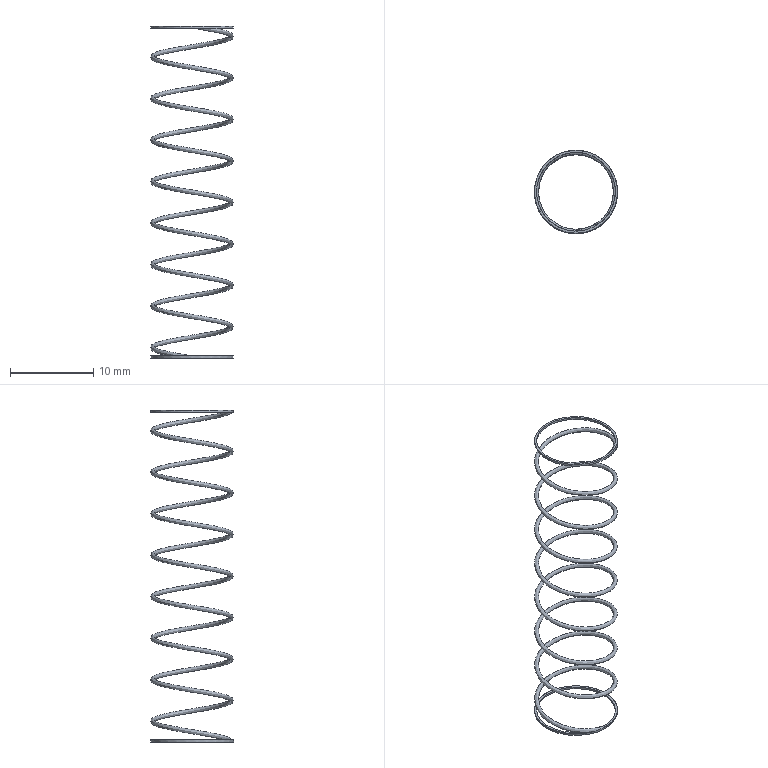Part | NX | features MFD10-WL40_2 2 | 1 solid | 11 faces | box 10 x 10 x 40 mm | volume 50.656 mm3 | plane 6 | cylinder 4 | spline 1 | commonest cylinder face diameters 9.5 x2 10 x2